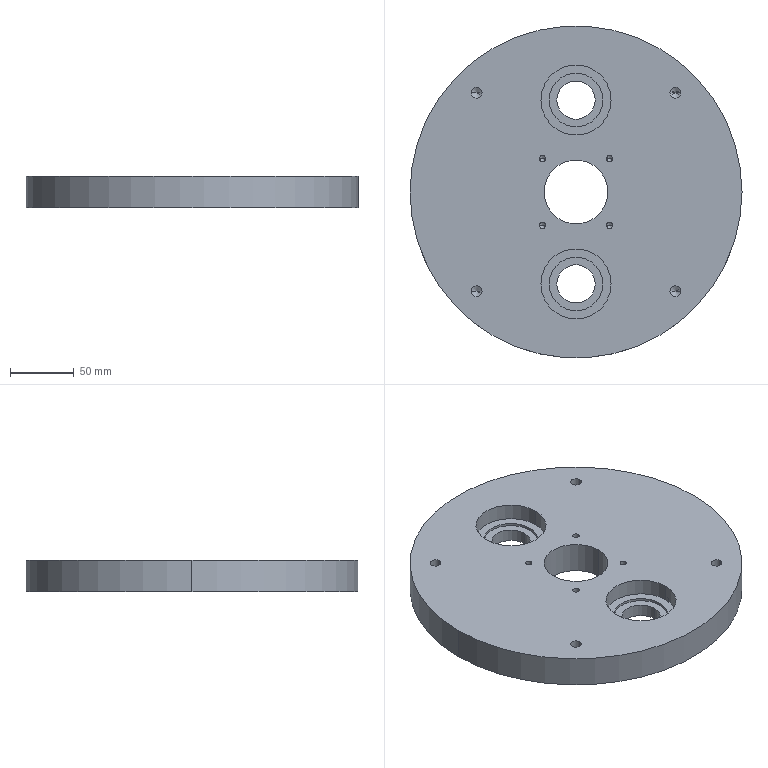Part | STEP file | Large pulley fixing disc SGN-2-08 | 1 solid | 70 faces | box 260 x 260 x 25 mm | volume 1189829 mm3 | cylinder 40 | cone 24 | plane 6 | commonest cylinder face diameters 5 x12 8.5 x8 6.8 x4 30 x4 42 x4 55 x4